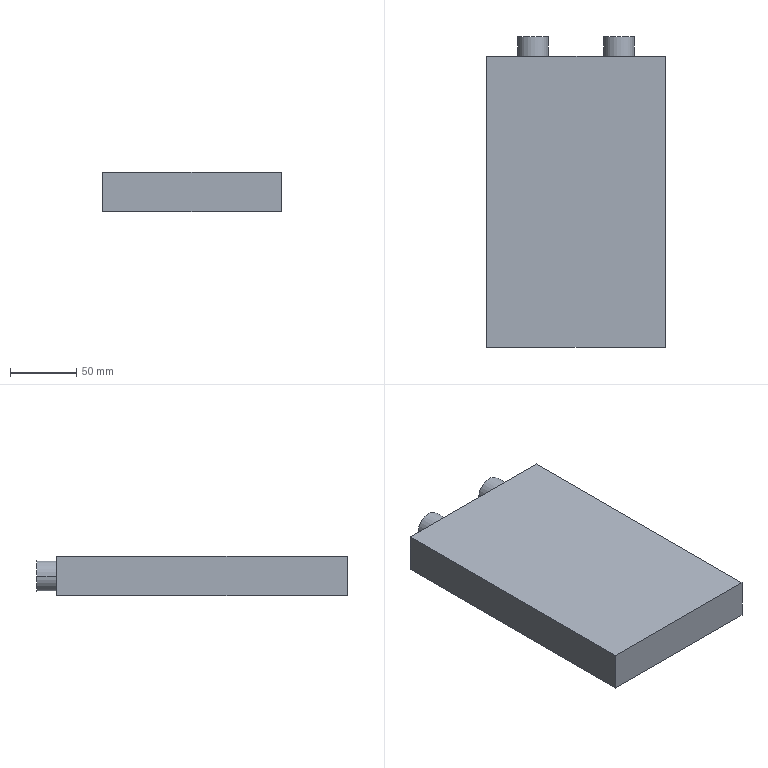Part | SolidWorks | features Extrusion 1, ICE 1 | 1 solid | 12 faces | box 135 x 235 x 30 mm | volume 903464 mm3 | plane 8 | cylinder 4 | commonest cylinder face diameters 23 x4
STEP:
#1=CARTESIAN_POINT('',(-44.,125.,0.));
#2=VERTEX_POINT('',#1);
#3=CARTESIAN_POINT('',(-21.,125.,0.));
#4=VERTEX_POINT('',#3);
#5=CARTESIAN_POINT('',(-32.5,125.,0.));
#6=DIRECTION('',(0.,1.,0.));
#7=DIRECTION('',(-1.,0.,0.));
#8=AXIS2_PLACEMENT_3D('',#5,#6,#7);
#9=CIRCLE('',#8,11.5);
#10=EDGE_CURVE('',#2,#4,#9,.T.);
#11=ORIENTED_EDGE('',*,*,#10,.F.);
#12=CARTESIAN_POINT('',(-44.,110.,0.));
#13=VERTEX_POINT('',#12);
#14=CARTESIAN_POINT('',(-44.,125.,0.));
#15=DIRECTION('',(0.,-1.,0.));
#16=VECTOR('',#15,1000.);
#17=LINE('',#14,#16);
#18=EDGE_CURVE('',#2,#13,#17,.T.);
#19=ORIENTED_EDGE('',*,*,#18,.T.);
#20=CARTESIAN_POINT('',(-21.,110.,0.));
#21=VERTEX_POINT('',#20);
#22=CARTESIAN_POINT('',(-32.5,110.,0.));
#23=DIRECTION('',(0.,1.,0.));
#24=DIRECTION('',(1.,0.,0.));
#25=AXIS2_PLACEMENT_3D('',#22,#23,#24);
#26=CIRCLE('',#25,11.5);
#27=EDGE_CURVE('',#13,#21,#26,.T.);
#28=ORIENTED_EDGE('',*,*,#27,.T.);
#29=CARTESIAN_POINT('',(-21.,125.,0.));
#30=DIRECTION('',(0.,-1.,0.));
#31=VECTOR('',#30,1000.);
#32=LINE('',#29,#31);
#33=EDGE_CURVE('',#4,#21,#32,.T.);
#34=ORIENTED_EDGE('',*,*,#33,.F.);
#35=EDGE_LOOP('',(#11,#19,#28,#34));
#36=FACE_OUTER_BOUND('',#35,.T.);
#37=CARTESIAN_POINT('',(-32.5,125.,0.));
#38=DIRECTION('',(0.,-1.,0.));
#39=DIRECTION('',(1.,0.,0.));
#40=AXIS2_PLACEMENT_3D('',#37,#38,#39);
#41=CYLINDRICAL_SURFACE('',#40,11.5);
#42=ADVANCED_FACE('',(#36),#41,.T.);
#43=CARTESIAN_POINT('',(21.,125.,0.));
#44=VERTEX_POINT('',#43);
#45=CARTESIAN_POINT('',(44.,125.,0.));
#46=VERTEX_POINT('',#45);
#47=CARTESIAN_POINT('',(32.5,125.,0.));
#48=DIRECTION('',(0.,1.,0.));
#49=DIRECTION('',(-1.,0.,0.));
#50=AXIS2_PLACEMENT_3D('',#47,#48,#49);
#51=CIRCLE('',#50,11.5);
#52=EDGE_CURVE('',#44,#46,#51,.T.);
#53=ORIENTED_EDGE('',*,*,#52,.F.);
#54=CARTESIAN_POINT('',(21.,110.,0.));
#55=VERTEX_POINT('',#54);
#56=CARTESIAN_POINT('',(21.,125.,0.));
#57=DIRECTION('',(0.,-1.,0.));
#58=VECTOR('',#57,1000.);
#59=LINE('',#56,#58);
#60=EDGE_CURVE('',#44,#55,#59,.T.);
#61=ORIENTED_EDGE('',*,*,#60,.T.);
#62=CARTESIAN_POINT('',(44.,110.,0.));
#63=VERTEX_POINT('',#62);
#64=CARTESIAN_POINT('',(32.5,110.,0.));
#65=DIRECTION('',(0.,1.,0.));
#66=DIRECTION('',(1.,0.,0.));
#67=AXIS2_PLACEMENT_3D('',#64,#65,#66);
#68=CIRCLE('',#67,11.5);
#69=EDGE_CURVE('',#55,#63,#68,.T.);
#70=ORIENTED_EDGE('',*,*,#69,.T.);
#71=CARTESIAN_POINT('',(44.,125.,0.));
#72=DIRECTION('',(0.,-1.,0.));
#73=VECTOR('',#72,1000.);
#74=LINE('',#71,#73);
#75=EDGE_CURVE('',#46,#63,#74,.T.);
#76=ORIENTED_EDGE('',*,*,#75,.F.);
#77=EDGE_LOOP('',(#53,#61,#70,#76));
#78=FACE_OUTER_BOUND('',#77,.T.);
#79=CARTESIAN_POINT('',(32.5,125.,0.));
#80=DIRECTION('',(0.,-1.,0.));
#81=DIRECTION('',(1.,0.,0.));
#82=AXIS2_PLACEMENT_3D('',#79,#80,#81);
#83=CYLINDRICAL_SURFACE('',#82,11.5);
#84=ADVANCED_FACE('',(#78),#83,.T.);
#85=CARTESIAN_POINT('',(67.5,110.,-15.));
#86=VERTEX_POINT('',#85);
#87=CARTESIAN_POINT('',(-67.5,110.,-15.));
#88=VERTEX_POINT('',#87);
#89=CARTESIAN_POINT('',(-67.5,110.,-15.));
#90=DIRECTION('',(-1.,0.,0.));
#91=VECTOR('',#90,1000.);
#92=LINE('',#89,#91);
#93=EDGE_CURVE('',#86,#88,#92,.T.);
#94=ORIENTED_EDGE('',*,*,#93,.T.);
#95=CARTESIAN_POINT('',(-67.5,110.,15.));
#96=VERTEX_POINT('',#95);
#97=CARTESIAN_POINT('',(-67.5,110.,15.));
#98=DIRECTION('',(0.,0.,-1.));
#99=VECTOR('',#98,1000.);
#100=LINE('',#97,#99);
#101=EDGE_CURVE('',#96,#88,#100,.T.);
#102=ORIENTED_EDGE('',*,*,#101,.F.);
#103=CARTESIAN_POINT('',(67.5,110.,15.));
#104=VERTEX_POINT('',#103);
#105=CARTESIAN_POINT('',(-67.5,110.,15.));
#106=DIRECTION('',(-1.,0.,0.));
#107=VECTOR('',#106,1000.);
#108=LINE('',#105,#107);
#109=EDGE_CURVE('',#104,#96,#108,.T.);
#110=ORIENTED_EDGE('',*,*,#109,.F.);
#111=CARTESIAN_POINT('',(67.5,110.,15.));
#112=DIRECTION('',(0.,0.,-1.));
#113=VECTOR('',#112,1000.);
#114=LINE('',#111,#113);
#115=EDGE_CURVE('',#104,#86,#114,.T.);
#116=ORIENTED_EDGE('',*,*,#115,.T.);
#117=EDGE_LOOP('',(#94,#102,#110,#116));
#118=FACE_OUTER_BOUND('',#117,.T.);
#119=CARTESIAN_POINT('',(32.5,110.,0.));
#120=DIRECTION('',(0.,1.,0.));
#121=DIRECTION('',(1.,0.,0.));
#122=AXIS2_PLACEMENT_3D('',#119,#120,#121);
#123=CIRCLE('',#122,11.5);
#124=EDGE_CURVE('',#63,#55,#123,.T.);
#125=ORIENTED_EDGE('',*,*,#124,.F.);
#126=ORIENTED_EDGE('',*,*,#69,.F.);
#127=EDGE_LOOP('',(#125,#126));
#128=FACE_BOUND('',#127,.T.);
#129=CARTESIAN_POINT('',(-32.5,110.,0.));
#130=DIRECTION('',(0.,1.,0.));
#131=DIRECTION('',(1.,0.,0.));
#132=AXIS2_PLACEMENT_3D('',#129,#130,#131);
#133=CIRCLE('',#132,11.5);
#134=EDGE_CURVE('',#21,#13,#133,.T.);
#135=ORIENTED_EDGE('',*,*,#134,.F.);
#136=ORIENTED_EDGE('',*,*,#27,.F.);
#137=EDGE_LOOP('',(#135,#136));
#138=FACE_BOUND('',#137,.T.);
#139=CARTESIAN_POINT('',(-67.5,110.,15.));
#140=DIRECTION('',(0.,-1.,0.));
#141=DIRECTION('',(1.,0.,0.));
#142=AXIS2_PLACEMENT_3D('',#139,#140,#141);
#143=PLANE('',#142);
#144=ADVANCED_FACE('',(#118,#128,#138),#143,.F.);
#145=CARTESIAN_POINT('',(-67.5,-110.,-15.));
#146=VERTEX_POINT('',#145);
#147=CARTESIAN_POINT('',(-67.5,110.,-15.));
#148=DIRECTION('',(0.,-1.,0.));
#149=VECTOR('',#148,1000.);
#150=LINE('',#147,#149);
#151=EDGE_CURVE('',#88,#146,#150,.T.);
#152=ORIENTED_EDGE('',*,*,#151,.T.);
#153=CARTESIAN_POINT('',(-67.5,-110.,15.));
#154=VERTEX_POINT('',#153);
#155=CARTESIAN_POINT('',(-67.5,-110.,15.));
#156=DIRECTION('',(0.,0.,-1.));
#157=VECTOR('',#156,1000.);
#158=LINE('',#155,#157);
#159=EDGE_CURVE('',#154,#146,#158,.T.);
#160=ORIENTED_EDGE('',*,*,#159,.F.);
#161=CARTESIAN_POINT('',(-67.5,110.,15.));
#162=DIRECTION('',(0.,-1.,0.));
#163=VECTOR('',#162,1000.);
#164=LINE('',#161,#163);
#165=EDGE_CURVE('',#96,#154,#164,.T.);
#166=ORIENTED_EDGE('',*,*,#165,.F.);
#167=ORIENTED_EDGE('',*,*,#101,.T.);
#168=EDGE_LOOP('',(#152,#160,#166,#167));
#169=FACE_OUTER_BOUND('',#168,.T.);
#170=CARTESIAN_POINT('',(-67.5,110.,15.));
#171=DIRECTION('',(1.,0.,0.));
#172=DIRECTION('',(0.,0.,-1.));
#173=AXIS2_PLACEMENT_3D('',#170,#171,#172);
#174=PLANE('',#173);
#175=ADVANCED_FACE('',(#169),#174,.F.);
#176=CARTESIAN_POINT('',(67.5,-110.,-15.));
#177=VERTEX_POINT('',#176);
#178=CARTESIAN_POINT('',(-67.5,-110.,-15.));
#179=DIRECTION('',(1.,0.,0.));
#180=VECTOR('',#179,1000.);
#181=LINE('',#178,#180);
#182=EDGE_CURVE('',#146,#177,#181,.T.);
#183=ORIENTED_EDGE('',*,*,#182,.T.);
#184=CARTESIAN_POINT('',(67.5,-110.,15.));
#185=VERTEX_POINT('',#184);
#186=CARTESIAN_POINT('',(67.5,-110.,15.));
#187=DIRECTION('',(0.,0.,-1.));
#188=VECTOR('',#187,1000.);
#189=LINE('',#186,#188);
#190=EDGE_CURVE('',#185,#177,#189,.T.);
#191=ORIENTED_EDGE('',*,*,#190,.F.);
#192=CARTESIAN_POINT('',(-67.5,-110.,15.));
#193=DIRECTION('',(1.,0.,0.));
#194=VECTOR('',#193,1000.);
#195=LINE('',#192,#194);
#196=EDGE_CURVE('',#154,#185,#195,.T.);
#197=ORIENTED_EDGE('',*,*,#196,.F.);
#198=ORIENTED_EDGE('',*,*,#159,.T.);
#199=EDGE_LOOP('',(#183,#191,#197,#198));
#200=FACE_OUTER_BOUND('',#199,.T.);
#201=CARTESIAN_POINT('',(-67.5,-110.,15.));
#202=DIRECTION('',(0.,1.,0.));
#203=DIRECTION('',(-1.,0.,0.));
#204=AXIS2_PLACEMENT_3D('',#201,#202,#203);
#205=PLANE('',#204);
#206=ADVANCED_FACE('',(#200),#205,.F.);
#207=CARTESIAN_POINT('',(67.5,110.,-15.));
#208=DIRECTION('',(0.,1.,0.));
#209=VECTOR('',#208,1000.);
#210=LINE('',#207,#209);
#211=EDGE_CURVE('',#177,#86,#210,.T.);
#212=ORIENTED_EDGE('',*,*,#211,.T.);
#213=ORIENTED_EDGE('',*,*,#115,.F.);
#214=CARTESIAN_POINT('',(67.5,110.,15.));
#215=DIRECTION('',(0.,1.,0.));
#216=VECTOR('',#215,1000.);
#217=LINE('',#214,#216);
#218=EDGE_CURVE('',#185,#104,#217,.T.);
#219=ORIENTED_EDGE('',*,*,#218,.F.);
#220=ORIENTED_EDGE('',*,*,#190,.T.);
#221=EDGE_LOOP('',(#212,#213,#219,#220));
#222=FACE_OUTER_BOUND('',#221,.T.);
#223=CARTESIAN_POINT('',(67.5,110.,15.));
#224=DIRECTION('',(-1.,0.,0.));
#225=DIRECTION('',(0.,-1.,0.));
#226=AXIS2_PLACEMENT_3D('',#223,#224,#225);
#227=PLANE('',#226);
#228=ADVANCED_FACE('',(#222),#227,.F.);
#229=ORIENTED_EDGE('',*,*,#165,.T.);
#230=ORIENTED_EDGE('',*,*,#196,.T.);
#231=ORIENTED_EDGE('',*,*,#218,.T.);
#232=ORIENTED_EDGE('',*,*,#109,.T.);
#233=EDGE_LOOP('',(#229,#230,#231,#232));
#234=FACE_OUTER_BOUND('',#233,.T.);
#235=CARTESIAN_POINT('',(0.,0.,15.));
#236=DIRECTION('',(0.,0.,1.));
#237=DIRECTION('',(1.,0.,0.));
#238=AXIS2_PLACEMENT_3D('',#235,#236,#237);
#239=PLANE('',#238);
#240=ADVANCED_FACE('',(#234),#239,.T.);
#241=ORIENTED_EDGE('',*,*,#151,.F.);
#242=ORIENTED_EDGE('',*,*,#93,.F.);
#243=ORIENTED_EDGE('',*,*,#211,.F.);
#244=ORIENTED_EDGE('',*,*,#182,.F.);
#245=EDGE_LOOP('',(#241,#242,#243,#244));
#246=FACE_OUTER_BOUND('',#245,.T.);
#247=CARTESIAN_POINT('',(0.,0.,-15.));
#248=DIRECTION('',(0.,0.,1.));
#249=DIRECTION('',(1.,0.,0.));
#250=AXIS2_PLACEMENT_3D('',#247,#248,#249);
#251=PLANE('',#250);
#252=ADVANCED_FACE('',(#246),#251,.F.);
#253=ORIENTED_EDGE('',*,*,#60,.F.);
#254=CARTESIAN_POINT('',(32.5,125.,0.));
#255=DIRECTION('',(0.,1.,0.));
#256=DIRECTION('',(-1.,0.,0.));
#257=AXIS2_PLACEMENT_3D('',#254,#255,#256);
#258=CIRCLE('',#257,11.5);
#259=EDGE_CURVE('',#46,#44,#258,.T.);
#260=ORIENTED_EDGE('',*,*,#259,.F.);
#261=ORIENTED_EDGE('',*,*,#75,.T.);
#262=ORIENTED_EDGE('',*,*,#124,.T.);
#263=EDGE_LOOP('',(#253,#260,#261,#262));
#264=FACE_OUTER_BOUND('',#263,.T.);
#265=CARTESIAN_POINT('',(32.5,125.,0.));
#266=DIRECTION('',(0.,-1.,0.));
#267=DIRECTION('',(1.,0.,0.));
#268=AXIS2_PLACEMENT_3D('',#265,#266,#267);
#269=CYLINDRICAL_SURFACE('',#268,11.5);
#270=ADVANCED_FACE('',(#264),#269,.T.);
#271=ORIENTED_EDGE('',*,*,#259,.T.);
#272=ORIENTED_EDGE('',*,*,#52,.T.);
#273=EDGE_LOOP('',(#271,#272));
#274=FACE_OUTER_BOUND('',#273,.T.);
#275=CARTESIAN_POINT('',(32.5,125.,0.));
#276=DIRECTION('',(0.,1.,0.));
#277=DIRECTION('',(-1.,0.,0.));
#278=AXIS2_PLACEMENT_3D('',#275,#276,#277);
#279=PLANE('',#278);
#280=ADVANCED_FACE('',(#274),#279,.T.);
#281=ORIENTED_EDGE('',*,*,#18,.F.);
#282=CARTESIAN_POINT('',(-32.5,125.,0.));
#283=DIRECTION('',(0.,1.,0.));
#284=DIRECTION('',(-1.,0.,0.));
#285=AXIS2_PLACEMENT_3D('',#282,#283,#284);
#286=CIRCLE('',#285,11.5);
#287=EDGE_CURVE('',#4,#2,#286,.T.);
#288=ORIENTED_EDGE('',*,*,#287,.F.);
#289=ORIENTED_EDGE('',*,*,#33,.T.);
#290=ORIENTED_EDGE('',*,*,#134,.T.);
#291=EDGE_LOOP('',(#281,#288,#289,#290));
#292=FACE_OUTER_BOUND('',#291,.T.);
#293=CARTESIAN_POINT('',(-32.5,125.,0.));
#294=DIRECTION('',(0.,-1.,0.));
#295=DIRECTION('',(1.,0.,0.));
#296=AXIS2_PLACEMENT_3D('',#293,#294,#295);
#297=CYLINDRICAL_SURFACE('',#296,11.5);
#298=ADVANCED_FACE('',(#292),#297,.T.);
#299=ORIENTED_EDGE('',*,*,#287,.T.);
#300=ORIENTED_EDGE('',*,*,#10,.T.);
#301=EDGE_LOOP('',(#299,#300));
#302=FACE_OUTER_BOUND('',#301,.T.);
#303=CARTESIAN_POINT('',(-32.5,125.,0.));
#304=DIRECTION('',(0.,1.,0.));
#305=DIRECTION('',(-1.,0.,0.));
#306=AXIS2_PLACEMENT_3D('',#303,#304,#305);
#307=PLANE('',#306);
#308=ADVANCED_FACE('',(#302),#307,.T.);
#309=CLOSED_SHELL('',(#42,#84,#144,#175,#206,#228,#240,#252,#270,#280,#298,#308));
#310=MANIFOLD_SOLID_BREP('',#309);
#311=CARTESIAN_POINT('',(0.,0.,0.));
#312=DIRECTION('',(0.,0.,1.));
#313=DIRECTION('',(1.,0.,0.));
#314=AXIS2_PLACEMENT_3D('',#311,#312,#313);
#315=(LENGTH_UNIT()NAMED_UNIT(*)SI_UNIT(.MILLI.,.METRE.));
#316=UNCERTAINTY_MEASURE_WITH_UNIT(LENGTH_MEASURE(0.00001),#315,'','');
#317=(NAMED_UNIT(*)PLANE_ANGLE_UNIT()SI_UNIT($,.RADIAN.));
#318=(NAMED_UNIT(*)SI_UNIT($,.STERADIAN.)SOLID_ANGLE_UNIT());
#319=(GEOMETRIC_REPRESENTATION_CONTEXT(3)GLOBAL_UNCERTAINTY_ASSIGNED_CONTEXT((#316))GLOBAL_UNIT_ASSIGNED_CONTEXT((#315,#317,#318))REPRESENTATION_CONTEXT('',''));
#320=ADVANCED_BREP_SHAPE_REPRESENTATION('',(#310,#314),#319);